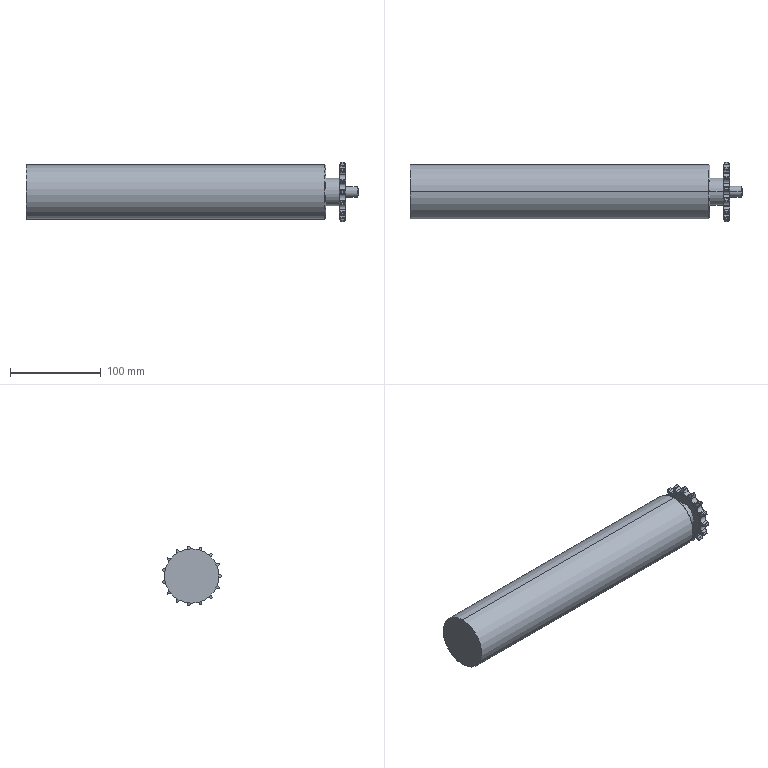Part | STEP file | Single sprocket roller_08B | 1 solid | 186 faces | box 365.5 x 65.419 x 65.772 mm | volume 961298 mm3 | cylinder 106 | plane 40 | spline 36 | cone 4 | commonest cylinder face diameters 12.509 x31 22.269 x31 8.653 x19 66 x15 8 x4 12 x2